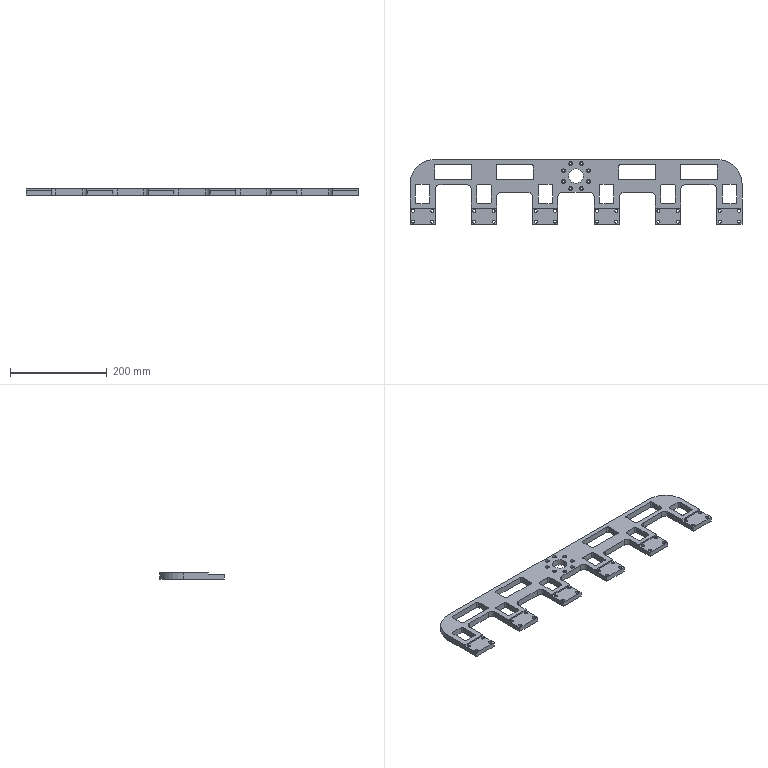CAM job | NX | 3-axis milling, drilling | part box 687 x 134 x 13 mm | stock box 691 x 138 x 14 mm
Tools:
number,name,description,diameter,corner_radius,flute_length,length,flutes
1,D63,Milling Tool-5 Parameters,63.0,0.0,50.0,75.0,2
7,D6A45,Milling Tool-5 Parameters,6.0,0.0,50.0,75.0,2
14,4.5ZT,Drilling Tool,4.5,0.0,35.0,50.0,2
15,6.5ZT,Drilling Tool,6.5,0.0,35.0,50.0,2
10,D10,Milling Tool-5 Parameters,10.0,0.0,50.0,75.0,2
Operations:
program,operation,operation_type,tool,method,geometry_group,spindle_rpm,surface_speed,feed_per_tooth,feed_cut,feed_plunge,cut_length_mm,path_length_mm,cut_time_min,machine_time_min
1,FLOOR_WALL_COPY,VolumeBased25DMillingOperation,D63,METHOD,A,6500.0,1286.0,0.1154,1500.0,100.0,3894.796,3948.796,2.596,2.602
1,DRILLING_COPY_1,Operation,D6A45,METHOD,A,5000.0,94.0,0.025,250.0,0.0,132.0,1577.891,0.528,0.6726
1,DRILLING_COPY_COPY_1,Operation,4.5ZT,METHOD,A,2000.0,28.0,0.0625,250.0,0.0,140.0,512.475,0.56,0.5972
1,DRILLING_COPY_COPY_COPY,Operation,6.5ZT,METHOD,A,2000.0,28.0,0.0625,250.0,0.0,420.0,1911.376,1.68,1.829
1,ZLEVEL_PROFILE_COPY_3,ZLevelMilling,D10,METHOD,A,9500.0,298.0,0.1842,3500.0,1000.0,32481.721,32552.721,9.315,9.322
1,ZLEVEL_PROFILE_COPY_2_COPY_COPY,ZLevelMilling,D10,METHOD,A,9500.0,298.0,0.1053,2000.0,1000.0,14258.066,17362.024,7.388,7.698
1,ZLEVEL_PROFILE_COPY_2_COPY,ZLevelMilling,D10,METHOD,A,9500.0,298.0,0.1842,3500.0,1000.0,20260.543,22700.982,6.159,6.403
1,ZLEVEL_PROFILE_COPY_COPY_1,ZLevelMilling,D10,METHOD,A,9500.0,298.0,0.0789,1500.0,1000.0,4862.944,8981.973,3.622,4.034
1,FLOOR_WALL_1_COPY_1,VolumeBased25DMillingOperation,D10,METHOD,A,9500.0,298.0,0.1579,3000.0,1000.0,9172.699,10386.251,3.088,3.209
1,FLOOR_WALL_1_COPY_COPY,VolumeBased25DMillingOperation,D10,METHOD,A,9500.0,298.0,0.0789,1500.0,1000.0,2508.515,3582.4,1.683,1.79
1,PLANAR_MILL_COPY_1,PlanarMilling,D6A45,METHOD,A,9500.0,179.0,0.0737,1400.0,100.0,3624.587,5261.27,2.589,2.753
1,PLANAR_MILL_COPY_COPY,PlanarMilling,D6A45,METHOD,A,9500.0,179.0,0.0737,1400.0,100.0,1198.131,5039.762,0.8558,1.24
1,ZLEVEL_PROFILE_COPY_3_COPY,ZLevelMilling,D10,METHOD,A,9500.0,298.0,0.0632,1200.0,1000.0,14142.838,14205.638,11.828,11.834